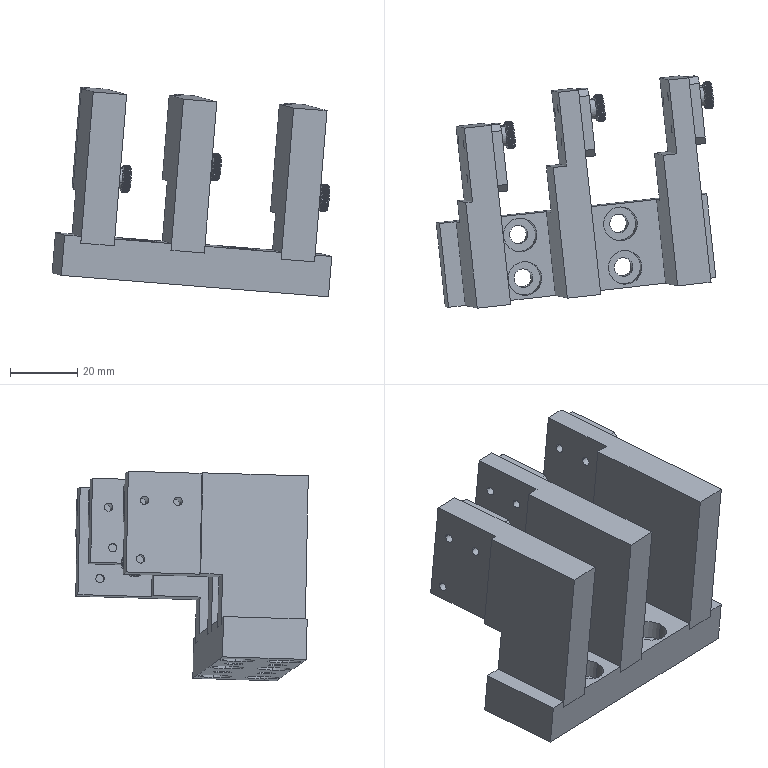Part | SolidWorks | 10 solids | 621 faces | box 82.95 x 68.99 x 62.182 mm | volume 75184 mm3 | plane 487 | cylinder 104 | cone 30 | commonest cylinder face diameters 5.5 x20 10 x20 2.5 x18 3.4 x18 4.2 x12 3 x10